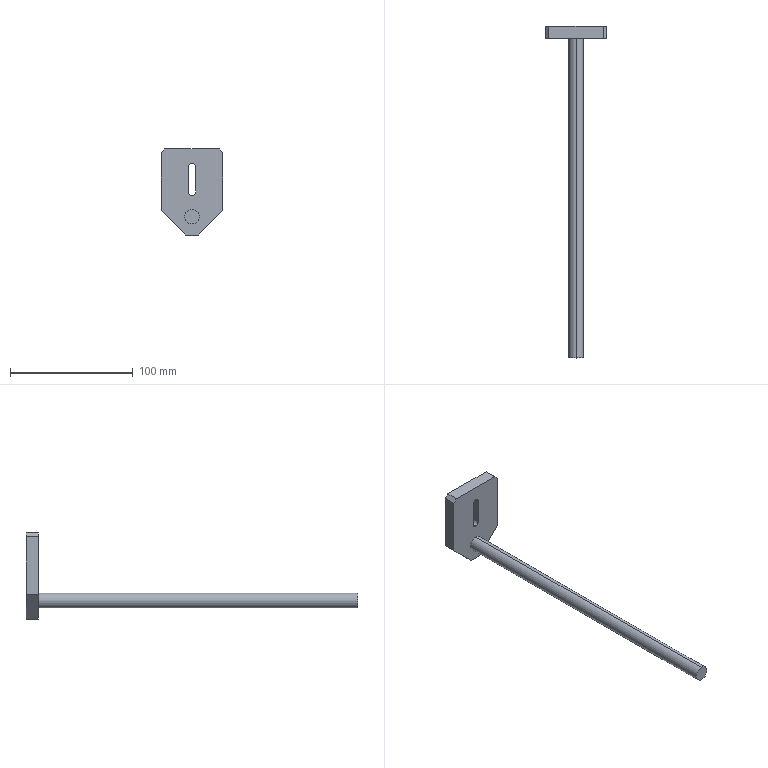Part | SolidWorks | features ICE 2, Chamfer 1, Extrusion 1, HoleWzd 1 | 1 solid | 20 faces | box 50 x 270 x 70 mm | volume 58386 mm3 | plane 13 | cylinder 7 | commonest cylinder face diameters 6 x3 4.2 x2 12 x2
STEP:
#1=CARTESIAN_POINT('',(0.,10.,-13.));
#2=VERTEX_POINT('',#1);
#3=CARTESIAN_POINT('',(3.,10.,-10.));
#4=VERTEX_POINT('',#3);
#5=CARTESIAN_POINT('',(0.,10.,-10.));
#6=DIRECTION('',(0.,-1.,0.));
#7=DIRECTION('',(0.,0.,-1.));
#8=AXIS2_PLACEMENT_3D('',#5,#6,#7);
#9=CIRCLE('',#8,3.);
#10=EDGE_CURVE('',#2,#4,#9,.T.);
#11=ORIENTED_EDGE('',*,*,#10,.F.);
#12=CARTESIAN_POINT('',(0.,7.1,-13.));
#13=VERTEX_POINT('',#12);
#14=CARTESIAN_POINT('',(0.,10.,-13.));
#15=DIRECTION('',(0.,-1.,0.));
#16=VECTOR('',#15,1000.);
#17=LINE('',#14,#16);
#18=EDGE_CURVE('',#2,#13,#17,.T.);
#19=ORIENTED_EDGE('',*,*,#18,.T.);
#20=CARTESIAN_POINT('',(2.1,5.,-12.142));
#21=VERTEX_POINT('',#20);
#22=CARTESIAN_POINT('',(2.1,5.,-12.142));
#23=CARTESIAN_POINT('',(2.1,5.142,-12.142));
#24=CARTESIAN_POINT('',(2.085,5.286,-12.157));
#25=CARTESIAN_POINT('',(2.028,5.562,-12.211));
#26=CARTESIAN_POINT('',(1.986,5.695,-12.249));
#27=CARTESIAN_POINT('',(1.88,5.946,-12.339));
#28=CARTESIAN_POINT('',(1.816,6.063,-12.39));
#29=CARTESIAN_POINT('',(1.668,6.282,-12.495));
#30=CARTESIAN_POINT('',(1.583,6.386,-12.551));
#31=CARTESIAN_POINT('',(1.396,6.574,-12.657));
#32=CARTESIAN_POINT('',(1.295,6.659,-12.709));
#33=CARTESIAN_POINT('',(1.072,6.811,-12.804));
#34=CARTESIAN_POINT('',(0.9508,6.877,-12.848));
#35=CARTESIAN_POINT('',(0.6972,6.986,-12.921));
#36=CARTESIAN_POINT('',(0.5628,7.028,-12.95));
#37=CARTESIAN_POINT('',(0.2837,7.086,-12.99));
#38=CARTESIAN_POINT('',(0.1426,7.1,-13.));
#39=CARTESIAN_POINT('',(0.,7.1,-13.));
#40=B_SPLINE_CURVE_WITH_KNOTS('',3,(#22,#23,#24,#25,#26,#27,#28,#29,#30,#31,#32,#33,#34,#35,#36,#37,#38,#39),.UNSPECIFIED.,.F.,.F.,(4,2,2,2,2,2,2,2,4),(0.006811,0.007236,0.007662,0.008087,0.008512,0.008938,0.009363,0.009789,0.01021),.UNSPECIFIED.);
#41=EDGE_CURVE('',#21,#13,#40,.T.);
#42=ORIENTED_EDGE('',*,*,#41,.F.);
#43=CARTESIAN_POINT('',(0.,2.9,-13.));
#44=VERTEX_POINT('',#43);
#45=CARTESIAN_POINT('',(0.,2.9,-13.));
#46=CARTESIAN_POINT('',(0.1432,2.9,-13.));
#47=CARTESIAN_POINT('',(0.2844,2.914,-12.99));
#48=CARTESIAN_POINT('',(0.5628,2.972,-12.95));
#49=CARTESIAN_POINT('',(0.6977,3.014,-12.921));
#50=CARTESIAN_POINT('',(0.9516,3.123,-12.848));
#51=CARTESIAN_POINT('',(1.073,3.19,-12.804));
#52=CARTESIAN_POINT('',(1.295,3.342,-12.709));
#53=CARTESIAN_POINT('',(1.397,3.427,-12.657));
#54=CARTESIAN_POINT('',(1.679,3.711,-12.495));
#55=CARTESIAN_POINT('',(1.828,3.93,-12.383));
#56=CARTESIAN_POINT('',(1.987,4.308,-12.249));
#57=CARTESIAN_POINT('',(2.028,4.439,-12.211));
#58=CARTESIAN_POINT('',(2.085,4.715,-12.157));
#59=CARTESIAN_POINT('',(2.1,4.858,-12.142));
#60=CARTESIAN_POINT('',(2.1,5.,-12.142));
#61=B_SPLINE_CURVE_WITH_KNOTS('',3,(#45,#46,#47,#48,#49,#50,#51,#52,#53,#54,#55,#56,#57,#58,#59,#60),.UNSPECIFIED.,.F.,.F.,(4,2,2,2,2,2,2,4),(0.003408,0.003833,0.004259,0.004684,0.005109,0.00596,0.006386,0.006811),.UNSPECIFIED.);
#62=EDGE_CURVE('',#44,#21,#61,.T.);
#63=ORIENTED_EDGE('',*,*,#62,.F.);
#64=CARTESIAN_POINT('',(0.,0.,-13.));
#65=VERTEX_POINT('',#64);
#66=CARTESIAN_POINT('',(0.,10.,-13.));
#67=DIRECTION('',(0.,-1.,0.));
#68=VECTOR('',#67,1000.);
#69=LINE('',#66,#68);
#70=EDGE_CURVE('',#44,#65,#69,.T.);
#71=ORIENTED_EDGE('',*,*,#70,.T.);
#72=CARTESIAN_POINT('',(3.,0.,-10.));
#73=VERTEX_POINT('',#72);
#74=CARTESIAN_POINT('',(0.,0.,-10.));
#75=DIRECTION('',(0.,-1.,0.));
#76=DIRECTION('',(0.,0.,-1.));
#77=AXIS2_PLACEMENT_3D('',#74,#75,#76);
#78=CIRCLE('',#77,3.);
#79=EDGE_CURVE('',#65,#73,#78,.T.);
#80=ORIENTED_EDGE('',*,*,#79,.T.);
#81=CARTESIAN_POINT('',(3.,10.,-10.));
#82=DIRECTION('',(0.,-1.,0.));
#83=VECTOR('',#82,1000.);
#84=LINE('',#81,#83);
#85=EDGE_CURVE('',#4,#73,#84,.T.);
#86=ORIENTED_EDGE('',*,*,#85,.F.);
#87=EDGE_LOOP('',(#11,#19,#42,#63,#71,#80,#86));
#88=FACE_OUTER_BOUND('',#87,.T.);
#89=CARTESIAN_POINT('',(0.,10.,-10.));
#90=DIRECTION('',(0.,-1.,0.));
#91=DIRECTION('',(0.,0.,-1.));
#92=AXIS2_PLACEMENT_3D('',#89,#90,#91);
#93=CYLINDRICAL_SURFACE('',#92,3.);
#94=ADVANCED_FACE('',(#88),#93,.F.);
#95=CARTESIAN_POINT('',(-2.1,5.,-12.142));
#96=VERTEX_POINT('',#95);
#97=CARTESIAN_POINT('',(-2.1,5.,-12.142));
#98=CARTESIAN_POINT('',(-2.1,4.855,-12.142));
#99=CARTESIAN_POINT('',(-2.085,4.715,-12.157));
#100=CARTESIAN_POINT('',(-2.029,4.44,-12.21));
#101=CARTESIAN_POINT('',(-1.987,4.306,-12.249));
#102=CARTESIAN_POINT('',(-1.828,3.932,-12.383));
#103=CARTESIAN_POINT('',(-1.677,3.709,-12.497));
#104=CARTESIAN_POINT('',(-1.397,3.427,-12.657));
#105=CARTESIAN_POINT('',(-1.293,3.34,-12.71));
#106=CARTESIAN_POINT('',(-1.072,3.189,-12.805));
#107=CARTESIAN_POINT('',(-0.9538,3.124,-12.847));
#108=CARTESIAN_POINT('',(-0.7002,3.015,-12.92));
#109=CARTESIAN_POINT('',(-0.5641,2.972,-12.95));
#110=CARTESIAN_POINT('',(-0.2875,2.915,-12.989));
#111=CARTESIAN_POINT('',(-0.1435,2.9,-13.));
#112=CARTESIAN_POINT('',(0.,2.9,-13.));
#113=B_SPLINE_CURVE_WITH_KNOTS('',3,(#97,#98,#99,#100,#101,#102,#103,#104,#105,#106,#107,#108,#109,#110,#111,#112),.UNSPECIFIED.,.F.,.F.,(4,2,2,2,2,2,2,4),(0.,0.000426,0.000852,0.001704,0.00213,0.002556,0.002982,0.003408),.UNSPECIFIED.);
#114=EDGE_CURVE('',#96,#44,#113,.T.);
#115=ORIENTED_EDGE('',*,*,#114,.T.);
#116=ORIENTED_EDGE('',*,*,#62,.T.);
#117=CARTESIAN_POINT('',(2.1,5.,-45.));
#118=VERTEX_POINT('',#117);
#119=CARTESIAN_POINT('',(2.1,5.,-45.));
#120=DIRECTION('',(0.,0.,-1.));
#121=VECTOR('',#120,1000.);
#122=LINE('',#119,#121);
#123=EDGE_CURVE('',#21,#118,#122,.T.);
#124=ORIENTED_EDGE('',*,*,#123,.T.);
#125=CARTESIAN_POINT('',(-2.1,5.,-45.));
#126=VERTEX_POINT('',#125);
#127=CARTESIAN_POINT('',(0.,5.,-45.));
#128=DIRECTION('',(0.,0.,-1.));
#129=DIRECTION('',(-1.,0.,0.));
#130=AXIS2_PLACEMENT_3D('',#127,#128,#129);
#131=CIRCLE('',#130,2.1);
#132=EDGE_CURVE('',#118,#126,#131,.T.);
#133=ORIENTED_EDGE('',*,*,#132,.T.);
#134=CARTESIAN_POINT('',(-2.1,5.,-45.));
#135=DIRECTION('',(0.,0.,-1.));
#136=VECTOR('',#135,1000.);
#137=LINE('',#134,#136);
#138=EDGE_CURVE('',#96,#126,#137,.T.);
#139=ORIENTED_EDGE('',*,*,#138,.F.);
#140=EDGE_LOOP('',(#115,#116,#124,#133,#139));
#141=FACE_OUTER_BOUND('',#140,.T.);
#142=CARTESIAN_POINT('',(0.,5.,-45.));
#143=DIRECTION('',(0.,0.,-1.));
#144=DIRECTION('',(-1.,0.,0.));
#145=AXIS2_PLACEMENT_3D('',#142,#143,#144);
#146=CYLINDRICAL_SURFACE('',#145,2.1);
#147=ADVANCED_FACE('',(#141),#146,.F.);
#148=CARTESIAN_POINT('',(0.,-260.,-36.));
#149=VERTEX_POINT('',#148);
#150=CARTESIAN_POINT('',(0.,-260.,-24.));
#151=VERTEX_POINT('',#150);
#152=CARTESIAN_POINT('',(0.,-260.,-30.));
#153=DIRECTION('',(0.,-1.,0.));
#154=DIRECTION('',(0.,0.,-1.));
#155=AXIS2_PLACEMENT_3D('',#152,#153,#154);
#156=CIRCLE('',#155,6.);
#157=EDGE_CURVE('',#149,#151,#156,.T.);
#158=ORIENTED_EDGE('',*,*,#157,.F.);
#159=CARTESIAN_POINT('',(0.,0.,-36.));
#160=VERTEX_POINT('',#159);
#161=CARTESIAN_POINT('',(0.,-260.,-36.));
#162=DIRECTION('',(0.,1.,0.));
#163=VECTOR('',#162,1000.);
#164=LINE('',#161,#163);
#165=EDGE_CURVE('',#149,#160,#164,.T.);
#166=ORIENTED_EDGE('',*,*,#165,.T.);
#167=CARTESIAN_POINT('',(0.,0.,-24.));
#168=VERTEX_POINT('',#167);
#169=CARTESIAN_POINT('',(0.,0.,-30.));
#170=DIRECTION('',(0.,-1.,0.));
#171=DIRECTION('',(0.,0.,1.));
#172=AXIS2_PLACEMENT_3D('',#169,#170,#171);
#173=CIRCLE('',#172,6.);
#174=EDGE_CURVE('',#160,#168,#173,.T.);
#175=ORIENTED_EDGE('',*,*,#174,.T.);
#176=CARTESIAN_POINT('',(0.,-260.,-24.));
#177=DIRECTION('',(0.,1.,0.));
#178=VECTOR('',#177,1000.);
#179=LINE('',#176,#178);
#180=EDGE_CURVE('',#151,#168,#179,.T.);
#181=ORIENTED_EDGE('',*,*,#180,.F.);
#182=EDGE_LOOP('',(#158,#166,#175,#181));
#183=FACE_OUTER_BOUND('',#182,.T.);
#184=CARTESIAN_POINT('',(0.,-260.,-30.));
#185=DIRECTION('',(0.,1.,0.));
#186=DIRECTION('',(0.,0.,1.));
#187=AXIS2_PLACEMENT_3D('',#184,#185,#186);
#188=CYLINDRICAL_SURFACE('',#187,6.);
#189=ADVANCED_FACE('',(#183),#188,.T.);
#190=CARTESIAN_POINT('',(25.,0.,-25.));
#191=VERTEX_POINT('',#190);
#192=CARTESIAN_POINT('',(5.,0.,-45.));
#193=VERTEX_POINT('',#192);
#194=CARTESIAN_POINT('',(5.,0.,-45.));
#195=DIRECTION('',(-0.7071,0.,-0.7071));
#196=VECTOR('',#195,1000.);
#197=LINE('',#194,#196);
#198=EDGE_CURVE('',#191,#193,#197,.T.);
#199=ORIENTED_EDGE('',*,*,#198,.T.);
#200=CARTESIAN_POINT('',(5.,10.,-45.));
#201=VERTEX_POINT('',#200);
#202=CARTESIAN_POINT('',(5.,10.,-45.));
#203=DIRECTION('',(0.,-1.,0.));
#204=VECTOR('',#203,1000.);
#205=LINE('',#202,#204);
#206=EDGE_CURVE('',#201,#193,#205,.T.);
#207=ORIENTED_EDGE('',*,*,#206,.F.);
#208=CARTESIAN_POINT('',(25.,10.,-25.));
#209=VERTEX_POINT('',#208);
#210=CARTESIAN_POINT('',(5.,10.,-45.));
#211=DIRECTION('',(-0.7071,0.,-0.7071));
#212=VECTOR('',#211,1000.);
#213=LINE('',#210,#212);
#214=EDGE_CURVE('',#209,#201,#213,.T.);
#215=ORIENTED_EDGE('',*,*,#214,.F.);
#216=CARTESIAN_POINT('',(25.,10.,-25.));
#217=DIRECTION('',(0.,-1.,0.));
#218=VECTOR('',#217,1000.);
#219=LINE('',#216,#218);
#220=EDGE_CURVE('',#209,#191,#219,.T.);
#221=ORIENTED_EDGE('',*,*,#220,.T.);
#222=EDGE_LOOP('',(#199,#207,#215,#221));
#223=FACE_OUTER_BOUND('',#222,.T.);
#224=CARTESIAN_POINT('',(5.,10.,-45.));
#225=DIRECTION('',(-0.7071,0.,0.7071));
#226=DIRECTION('',(0.7071,0.,0.7071));
#227=AXIS2_PLACEMENT_3D('',#224,#225,#226);
#228=PLANE('',#227);
#229=ADVANCED_FACE('',(#223),#228,.F.);
#230=CARTESIAN_POINT('',(0.,5.,-45.));
#231=DIRECTION('',(0.,0.,-1.));
#232=DIRECTION('',(-1.,0.,0.));
#233=AXIS2_PLACEMENT_3D('',#230,#231,#232);
#234=CIRCLE('',#233,2.1);
#235=EDGE_CURVE('',#126,#118,#234,.T.);
#236=ORIENTED_EDGE('',*,*,#235,.F.);
#237=ORIENTED_EDGE('',*,*,#132,.F.);
#238=EDGE_LOOP('',(#236,#237));
#239=FACE_BOUND('',#238,.T.);
#240=CARTESIAN_POINT('',(-5.,0.,-45.));
#241=VERTEX_POINT('',#240);
#242=CARTESIAN_POINT('',(-5.,0.,-45.));
#243=DIRECTION('',(-1.,0.,0.));
#244=VECTOR('',#243,1000.);
#245=LINE('',#242,#244);
#246=EDGE_CURVE('',#193,#241,#245,.T.);
#247=ORIENTED_EDGE('',*,*,#246,.T.);
#248=CARTESIAN_POINT('',(-5.,10.,-45.));
#249=VERTEX_POINT('',#248);
#250=CARTESIAN_POINT('',(-5.,10.,-45.));
#251=DIRECTION('',(0.,-1.,0.));
#252=VECTOR('',#251,1000.);
#253=LINE('',#250,#252);
#254=EDGE_CURVE('',#249,#241,#253,.T.);
#255=ORIENTED_EDGE('',*,*,#254,.F.);
#256=CARTESIAN_POINT('',(-5.,10.,-45.));
#257=DIRECTION('',(-1.,0.,0.));
#258=VECTOR('',#257,1000.);
#259=LINE('',#256,#258);
#260=EDGE_CURVE('',#201,#249,#259,.T.);
#261=ORIENTED_EDGE('',*,*,#260,.F.);
#262=ORIENTED_EDGE('',*,*,#206,.T.);
#263=EDGE_LOOP('',(#247,#255,#261,#262));
#264=FACE_OUTER_BOUND('',#263,.T.);
#265=CARTESIAN_POINT('',(-5.,10.,-45.));
#266=DIRECTION('',(0.,0.,1.));
#267=DIRECTION('',(1.,0.,0.));
#268=AXIS2_PLACEMENT_3D('',#265,#266,#267);
#269=PLANE('',#268);
#270=ADVANCED_FACE('',(#239,#264),#269,.F.);
#271=CARTESIAN_POINT('',(-25.,0.,-25.));
#272=VERTEX_POINT('',#271);
#273=CARTESIAN_POINT('',(-25.,0.,-25.));
#274=DIRECTION('',(-0.7071,0.,0.7071));
#275=VECTOR('',#274,1000.);
#276=LINE('',#273,#275);
#277=EDGE_CURVE('',#241,#272,#276,.T.);
#278=ORIENTED_EDGE('',*,*,#277,.T.);
#279=CARTESIAN_POINT('',(-25.,10.,-25.));
#280=VERTEX_POINT('',#279);
#281=CARTESIAN_POINT('',(-25.,10.,-25.));
#282=DIRECTION('',(0.,-1.,0.));
#283=VECTOR('',#282,1000.);
#284=LINE('',#281,#283);
#285=EDGE_CURVE('',#280,#272,#284,.T.);
#286=ORIENTED_EDGE('',*,*,#285,.F.);
#287=CARTESIAN_POINT('',(-25.,10.,-25.));
#288=DIRECTION('',(-0.7071,0.,0.7071));
#289=VECTOR('',#288,1000.);
#290=LINE('',#287,#289);
#291=EDGE_CURVE('',#249,#280,#290,.T.);
#292=ORIENTED_EDGE('',*,*,#291,.F.);
#293=ORIENTED_EDGE('',*,*,#254,.T.);
#294=EDGE_LOOP('',(#278,#286,#292,#293));
#295=FACE_OUTER_BOUND('',#294,.T.);
#296=CARTESIAN_POINT('',(-25.,10.,-25.));
#297=DIRECTION('',(0.7071,0.,0.7071));
#298=DIRECTION('',(0.7071,0.,-0.7071));
#299=AXIS2_PLACEMENT_3D('',#296,#297,#298);
#300=PLANE('',#299);
#301=ADVANCED_FACE('',(#295),#300,.F.);
#302=CARTESIAN_POINT('',(-25.,0.,22.));
#303=VERTEX_POINT('',#302);
#304=CARTESIAN_POINT('',(-25.,0.,25.));
#305=DIRECTION('',(0.,0.,1.));
#306=VECTOR('',#305,1000.);
#307=LINE('',#304,#306);
#308=EDGE_CURVE('',#272,#303,#307,.T.);
#309=ORIENTED_EDGE('',*,*,#308,.T.);
#310=CARTESIAN_POINT('',(-25.,10.,22.));
#311=VERTEX_POINT('',#310);
#312=CARTESIAN_POINT('',(-25.,10.,22.));
#313=DIRECTION('',(0.,1.,0.));
#314=VECTOR('',#313,1000.);
#315=LINE('',#312,#314);
#316=EDGE_CURVE('',#303,#311,#315,.T.);
#317=ORIENTED_EDGE('',*,*,#316,.T.);
#318=CARTESIAN_POINT('',(-25.,10.,25.));
#319=DIRECTION('',(0.,0.,1.));
#320=VECTOR('',#319,1000.);
#321=LINE('',#318,#320);
#322=EDGE_CURVE('',#280,#311,#321,.T.);
#323=ORIENTED_EDGE('',*,*,#322,.F.);
#324=ORIENTED_EDGE('',*,*,#285,.T.);
#325=EDGE_LOOP('',(#309,#317,#323,#324));
#326=FACE_OUTER_BOUND('',#325,.T.);
#327=CARTESIAN_POINT('',(-25.,10.,25.));
#328=DIRECTION('',(1.,0.,0.));
#329=DIRECTION('',(0.,0.,-1.));
#330=AXIS2_PLACEMENT_3D('',#327,#328,#329);
#331=PLANE('',#330);
#332=ADVANCED_FACE('',(#326),#331,.F.);
#333=CARTESIAN_POINT('',(-22.,0.,25.));
#334=VERTEX_POINT('',#333);
#335=CARTESIAN_POINT('',(22.,0.,25.));
#336=VERTEX_POINT('',#335);
#337=CARTESIAN_POINT('',(-25.,0.,25.));
#338=DIRECTION('',(1.,0.,0.));
#339=VECTOR('',#338,1000.);
#340=LINE('',#337,#339);
#341=EDGE_CURVE('',#334,#336,#340,.T.);
#342=ORIENTED_EDGE('',*,*,#341,.T.);
#343=CARTESIAN_POINT('',(22.,10.,25.));
#344=VERTEX_POINT('',#343);
#345=CARTESIAN_POINT('',(22.,10.,25.));
#346=DIRECTION('',(0.,1.,0.));
#347=VECTOR('',#346,1000.);
#348=LINE('',#345,#347);
#349=EDGE_CURVE('',#336,#344,#348,.T.);
#350=ORIENTED_EDGE('',*,*,#349,.T.);
#351=CARTESIAN_POINT('',(-22.,10.,25.));
#352=VERTEX_POINT('',#351);
#353=CARTESIAN_POINT('',(-25.,10.,25.));
#354=DIRECTION('',(1.,0.,0.));
#355=VECTOR('',#354,1000.);
#356=LINE('',#353,#355);
#357=EDGE_CURVE('',#352,#344,#356,.T.);
#358=ORIENTED_EDGE('',*,*,#357,.F.);
#359=CARTESIAN_POINT('',(-22.,10.,25.));
#360=DIRECTION('',(0.,-1.,0.));
#361=VECTOR('',#360,1000.);
#362=LINE('',#359,#361);
#363=EDGE_CURVE('',#352,#334,#362,.T.);
#364=ORIENTED_EDGE('',*,*,#363,.T.);
#365=EDGE_LOOP('',(#342,#350,#358,#364));
#366=FACE_OUTER_BOUND('',#365,.T.);
#367=CARTESIAN_POINT('',(-25.,10.,25.));
#368=DIRECTION('',(0.,0.,-1.));
#369=DIRECTION('',(-1.,0.,0.));
#370=AXIS2_PLACEMENT_3D('',#367,#368,#369);
#371=PLANE('',#370);
#372=ADVANCED_FACE('',(#366),#371,.F.);
#373=CARTESIAN_POINT('',(25.,10.,22.));
#374=VERTEX_POINT('',#373);
#375=CARTESIAN_POINT('',(25.,10.,25.));
#376=DIRECTION('',(0.,0.,-1.));
#377=VECTOR('',#376,1000.);
#378=LINE('',#375,#377);
#379=EDGE_CURVE('',#374,#209,#378,.T.);
#380=ORIENTED_EDGE('',*,*,#379,.F.);
#381=CARTESIAN_POINT('',(25.,0.,22.));
#382=VERTEX_POINT('',#381);
#383=CARTESIAN_POINT('',(25.,10.,22.));
#384=DIRECTION('',(0.,-1.,0.));
#385=VECTOR('',#384,1000.);
#386=LINE('',#383,#385);
#387=EDGE_CURVE('',#374,#382,#386,.T.);
#388=ORIENTED_EDGE('',*,*,#387,.T.);
#389=CARTESIAN_POINT('',(25.,0.,25.));
#390=DIRECTION('',(0.,0.,-1.));
#391=VECTOR('',#390,1000.);
#392=LINE('',#389,#391);
#393=EDGE_CURVE('',#382,#191,#392,.T.);
#394=ORIENTED_EDGE('',*,*,#393,.T.);
#395=ORIENTED_EDGE('',*,*,#220,.F.);
#396=EDGE_LOOP('',(#380,#388,#394,#395));
#397=FACE_OUTER_BOUND('',#396,.T.);
#398=CARTESIAN_POINT('',(25.,10.,25.));
#399=DIRECTION('',(-1.,0.,0.));
#400=DIRECTION('',(0.,0.,1.));
#401=AXIS2_PLACEMENT_3D('',#398,#399,#400);
#402=PLANE('',#401);
#403=ADVANCED_FACE('',(#397),#402,.F.);
#404=CARTESIAN_POINT('',(3.,10.,10.));
#405=VERTEX_POINT('',#404);
#406=CARTESIAN_POINT('',(-3.,10.,10.));
#407=VERTEX_POINT('',#406);
#408=CARTESIAN_POINT('',(0.,10.,10.));
#409=DIRECTION('',(0.,-1.,0.));
#410=DIRECTION('',(0.,0.,-1.));
#411=AXIS2_PLACEMENT_3D('',#408,#409,#410);
#412=CIRCLE('',#411,3.);
#413=EDGE_CURVE('',#405,#407,#412,.T.);
#414=ORIENTED_EDGE('',*,*,#413,.T.);
#415=CARTESIAN_POINT('',(-3.,10.,-10.));
#416=VERTEX_POINT('',#415);
#417=CARTESIAN_POINT('',(-3.,10.,10.));
#418=DIRECTION('',(0.,0.,-1.));
#419=VECTOR('',#418,1000.);
#420=LINE('',#417,#419);
#421=EDGE_CURVE('',#407,#416,#420,.T.);
#422=ORIENTED_EDGE('',*,*,#421,.T.);
#423=CARTESIAN_POINT('',(0.,10.,-10.));
#424=DIRECTION('',(0.,-1.,0.));
#425=DIRECTION('',(0.,0.,-1.));
#426=AXIS2_PLACEMENT_3D('',#423,#424,#425);
#427=CIRCLE('',#426,3.);
#428=EDGE_CURVE('',#416,#2,#427,.T.);
#429=ORIENTED_EDGE('',*,*,#428,.T.);
#430=ORIENTED_EDGE('',*,*,#10,.T.);
#431=CARTESIAN_POINT('',(3.,10.,10.));
#432=DIRECTION('',(0.,0.,1.));
#433=VECTOR('',#432,1000.);
#434=LINE('',#431,#433);
#435=EDGE_CURVE('',#4,#405,#434,.T.);
#436=ORIENTED_EDGE('',*,*,#435,.T.);
#437=EDGE_LOOP('',(#414,#422,#429,#430,#436));
#438=FACE_BOUND('',#437,.T.);
#439=ORIENTED_EDGE('',*,*,#357,.T.);
#440=CARTESIAN_POINT('',(23.5,10.,23.5));
#441=DIRECTION('',(0.7071,0.,-0.7071));
#442=VECTOR('',#441,1000.);
#443=LINE('',#440,#442);
#444=EDGE_CURVE('',#344,#374,#443,.T.);
#445=ORIENTED_EDGE('',*,*,#444,.T.);
#446=ORIENTED_EDGE('',*,*,#379,.T.);
#447=ORIENTED_EDGE('',*,*,#214,.T.);
#448=ORIENTED_EDGE('',*,*,#260,.T.);
#449=ORIENTED_EDGE('',*,*,#291,.T.);
#450=ORIENTED_EDGE('',*,*,#322,.T.);
#451=CARTESIAN_POINT('',(-23.5,10.,23.5));
#452=DIRECTION('',(0.7071,0.,0.7071));
#453=VECTOR('',#452,1000.);
#454=LINE('',#451,#453);
#455=EDGE_CURVE('',#311,#352,#454,.T.);
#456=ORIENTED_EDGE('',*,*,#455,.T.);
#457=EDGE_LOOP('',(#439,#445,#446,#447,#448,#449,#450,#456));
#458=FACE_OUTER_BOUND('',#457,.T.);
#459=CARTESIAN_POINT('',(0.,10.,0.));
#460=DIRECTION('',(0.,1.,0.));
#461=DIRECTION('',(0.,0.,1.));
#462=AXIS2_PLACEMENT_3D('',#459,#460,#461);
#463=PLANE('',#462);
#464=ADVANCED_FACE('',(#438,#458),#463,.T.);
#465=CARTESIAN_POINT('',(-3.,0.,10.));
#466=VERTEX_POINT('',#465);
#467=CARTESIAN_POINT('',(-3.,0.,-10.));
#468=VERTEX_POINT('',#467);
#469=CARTESIAN_POINT('',(-3.,0.,10.));
#470=DIRECTION('',(0.,0.,-1.));
#471=VECTOR('',#470,1000.);
#472=LINE('',#469,#471);
#473=EDGE_CURVE('',#466,#468,#472,.T.);
#474=ORIENTED_EDGE('',*,*,#473,.F.);
#475=CARTESIAN_POINT('',(3.,0.,10.));
#476=VERTEX_POINT('',#475);
#477=CARTESIAN_POINT('',(0.,0.,10.));
#478=DIRECTION('',(0.,-1.,0.));
#479=DIRECTION('',(0.,0.,-1.));
#480=AXIS2_PLACEMENT_3D('',#477,#478,#479);
#481=CIRCLE('',#480,3.);
#482=EDGE_CURVE('',#476,#466,#481,.T.);
#483=ORIENTED_EDGE('',*,*,#482,.F.);
#484=CARTESIAN_POINT('',(3.,0.,10.));
#485=DIRECTION('',(0.,0.,1.));
#486=VECTOR('',#485,1000.);
#487=LINE('',#484,#486);
#488=EDGE_CURVE('',#73,#476,#487,.T.);
#489=ORIENTED_EDGE('',*,*,#488,.F.);
#490=ORIENTED_EDGE('',*,*,#79,.F.);
#491=CARTESIAN_POINT('',(0.,0.,-10.));
#492=DIRECTION('',(0.,-1.,0.));
#493=DIRECTION('',(0.,0.,-1.));
#494=AXIS2_PLACEMENT_3D('',#491,#492,#493);
#495=CIRCLE('',#494,3.);
#496=EDGE_CURVE('',#468,#65,#495,.T.);
#497=ORIENTED_EDGE('',*,*,#496,.F.);
#498=EDGE_LOOP('',(#474,#483,#489,#490,#497));
#499=FACE_BOUND('',#498,.T.);
#500=CARTESIAN_POINT('',(0.,0.,-30.));
#501=DIRECTION('',(0.,-1.,0.));
#502=DIRECTION('',(0.,0.,1.));
#503=AXIS2_PLACEMENT_3D('',#500,#501,#502);
#504=CIRCLE('',#503,6.);
#505=EDGE_CURVE('',#168,#160,#504,.T.);
#506=ORIENTED_EDGE('',*,*,#505,.F.);
#507=ORIENTED_EDGE('',*,*,#174,.F.);
#508=EDGE_LOOP('',(#506,#507));
#509=FACE_BOUND('',#508,.T.);
#510=ORIENTED_EDGE('',*,*,#393,.F.);
#511=CARTESIAN_POINT('',(25.,0.,22.));
#512=DIRECTION('',(-0.7071,0.,0.7071));
#513=VECTOR('',#512,1000.);
#514=LINE('',#511,#513);
#515=EDGE_CURVE('',#382,#336,#514,.T.);
#516=ORIENTED_EDGE('',*,*,#515,.T.);
#517=ORIENTED_EDGE('',*,*,#341,.F.);
#518=CARTESIAN_POINT('',(-22.,0.,25.));
#519=DIRECTION('',(-0.7071,0.,-0.7071));
#520=VECTOR('',#519,1000.);
#521=LINE('',#518,#520);
#522=EDGE_CURVE('',#334,#303,#521,.T.);
#523=ORIENTED_EDGE('',*,*,#522,.T.);
#524=ORIENTED_EDGE('',*,*,#308,.F.);
#525=ORIENTED_EDGE('',*,*,#277,.F.);
#526=ORIENTED_EDGE('',*,*,#246,.F.);
#527=ORIENTED_EDGE('',*,*,#198,.F.);
#528=EDGE_LOOP('',(#510,#516,#517,#523,#524,#525,#526,#527));
#529=FACE_OUTER_BOUND('',#528,.T.);
#530=CARTESIAN_POINT('',(0.,0.,0.));
#531=DIRECTION('',(0.,1.,0.));
#532=DIRECTION('',(0.,0.,1.));
#533=AXIS2_PLACEMENT_3D('',#530,#531,#532);
#534=PLANE('',#533);
#535=ADVANCED_FACE('',(#499,#509,#529),#534,.F.);
#536=ORIENTED_EDGE('',*,*,#165,.F.);
#537=CARTESIAN_POINT('',(0.,-260.,-30.));
#538=DIRECTION('',(0.,-1.,0.));
#539=DIRECTION('',(0.,0.,-1.));
#540=AXIS2_PLACEMENT_3D('',#537,#538,#539);
#541=CIRCLE('',#540,6.);
#542=EDGE_CURVE('',#151,#149,#541,.T.);
#543=ORIENTED_EDGE('',*,*,#542,.F.);
#544=ORIENTED_EDGE('',*,*,#180,.T.);
#545=ORIENTED_EDGE('',*,*,#505,.T.);
#546=EDGE_LOOP('',(#536,#543,#544,#545));
#547=FACE_OUTER_BOUND('',#546,.T.);
#548=CARTESIAN_POINT('',(0.,-260.,-30.));
#549=DIRECTION('',(0.,1.,0.));
#550=DIRECTION('',(0.,0.,1.));
#551=AXIS2_PLACEMENT_3D('',#548,#549,#550);
#552=CYLINDRICAL_SURFACE('',#551,6.);
#553=ADVANCED_FACE('',(#547),#552,.T.);
#554=ORIENTED_EDGE('',*,*,#542,.T.);
#555=ORIENTED_EDGE('',*,*,#157,.T.);
#556=EDGE_LOOP('',(#554,#555));
#557=FACE_OUTER_BOUND('',#556,.T.);
#558=CARTESIAN_POINT('',(0.,-260.,-30.));
#559=DIRECTION('',(0.,-1.,0.));
#560=DIRECTION('',(0.,0.,-1.));
#561=AXIS2_PLACEMENT_3D('',#558,#559,#560);
#562=PLANE('',#561);
#563=ADVANCED_FACE('',(#557),#562,.T.);
#564=ORIENTED_EDGE('',*,*,#123,.F.);
#565=ORIENTED_EDGE('',*,*,#41,.T.);
#566=CARTESIAN_POINT('',(0.,7.1,-13.));
#567=CARTESIAN_POINT('',(-0.1424,7.1,-13.));
#568=CARTESIAN_POINT('',(-0.2871,7.085,-12.989));
#569=CARTESIAN_POINT('',(-0.5634,7.028,-12.95));
#570=CARTESIAN_POINT('',(-0.6985,6.985,-12.921));
#571=CARTESIAN_POINT('',(-1.081,6.822,-12.811));
#572=CARTESIAN_POINT('',(-1.306,6.666,-12.709));
#573=CARTESIAN_POINT('',(-1.678,6.29,-12.496));
#574=CARTESIAN_POINT('',(-1.828,6.067,-12.382));
#575=CARTESIAN_POINT('',(-1.986,5.695,-12.249));
#576=CARTESIAN_POINT('',(-2.028,5.562,-12.211));
#577=CARTESIAN_POINT('',(-2.085,5.286,-12.157));
#578=CARTESIAN_POINT('',(-2.1,5.144,-12.142));
#579=CARTESIAN_POINT('',(-2.1,5.,-12.142));
#580=B_SPLINE_CURVE_WITH_KNOTS('',3,(#566,#567,#568,#569,#570,#571,#572,#573,#574,#575,#576,#577,#578,#579),.UNSPECIFIED.,.F.,.F.,(4,2,2,2,2,2,4),(0.01021,0.01064,0.01106,0.01191,0.01276,0.01319,0.01361),.UNSPECIFIED.);
#581=EDGE_CURVE('',#13,#96,#580,.T.);
#582=ORIENTED_EDGE('',*,*,#581,.T.);
#583=ORIENTED_EDGE('',*,*,#138,.T.);
#584=ORIENTED_EDGE('',*,*,#235,.T.);
#585=EDGE_LOOP('',(#564,#565,#582,#583,#584));
#586=FACE_OUTER_BOUND('',#585,.T.);
#587=CARTESIAN_POINT('',(0.,5.,-45.));
#588=DIRECTION('',(0.,0.,-1.));
#589=DIRECTION('',(-1.,0.,0.));
#590=AXIS2_PLACEMENT_3D('',#587,#588,#589);
#591=CYLINDRICAL_SURFACE('',#590,2.1);
#592=ADVANCED_FACE('',(#586),#591,.F.);
#593=ORIENTED_EDGE('',*,*,#18,.F.);
#594=ORIENTED_EDGE('',*,*,#428,.F.);
#595=CARTESIAN_POINT('',(-3.,10.,-10.));
#596=DIRECTION('',(0.,-1.,0.));
#597=VECTOR('',#596,1000.);
#598=LINE('',#595,#597);
#599=EDGE_CURVE('',#416,#468,#598,.T.);
#600=ORIENTED_EDGE('',*,*,#599,.T.);
#601=ORIENTED_EDGE('',*,*,#496,.T.);
#602=ORIENTED_EDGE('',*,*,#70,.F.);
#603=ORIENTED_EDGE('',*,*,#114,.F.);
#604=ORIENTED_EDGE('',*,*,#581,.F.);
#605=EDGE_LOOP('',(#593,#594,#600,#601,#602,#603,#604));
#606=FACE_OUTER_BOUND('',#605,.T.);
#607=CARTESIAN_POINT('',(0.,10.,-10.));
#608=DIRECTION('',(0.,-1.,0.));
#609=DIRECTION('',(0.,0.,-1.));
#610=AXIS2_PLACEMENT_3D('',#607,#608,#609);
#611=CYLINDRICAL_SURFACE('',#610,3.);
#612=ADVANCED_FACE('',(#606),#611,.F.);
#613=ORIENTED_EDGE('',*,*,#482,.T.);
#614=CARTESIAN_POINT('',(-3.,10.,10.));
#615=DIRECTION('',(0.,-1.,0.));
#616=VECTOR('',#615,1000.);
#617=LINE('',#614,#616);
#618=EDGE_CURVE('',#407,#466,#617,.T.);
#619=ORIENTED_EDGE('',*,*,#618,.F.);
#620=ORIENTED_EDGE('',*,*,#413,.F.);
#621=CARTESIAN_POINT('',(3.,10.,10.));
#622=DIRECTION('',(0.,-1.,0.));
#623=VECTOR('',#622,1000.);
#624=LINE('',#621,#623);
#625=EDGE_CURVE('',#405,#476,#624,.T.);
#626=ORIENTED_EDGE('',*,*,#625,.T.);
#627=EDGE_LOOP('',(#613,#619,#620,#626));
#628=FACE_OUTER_BOUND('',#627,.T.);
#629=CARTESIAN_POINT('',(0.,10.,10.));
#630=DIRECTION('',(0.,-1.,0.));
#631=DIRECTION('',(0.,0.,-1.));
#632=AXIS2_PLACEMENT_3D('',#629,#630,#631);
#633=CYLINDRICAL_SURFACE('',#632,3.);
#634=ADVANCED_FACE('',(#628),#633,.F.);
#635=ORIENTED_EDGE('',*,*,#488,.T.);
#636=ORIENTED_EDGE('',*,*,#625,.F.);
#637=ORIENTED_EDGE('',*,*,#435,.F.);
#638=ORIENTED_EDGE('',*,*,#85,.T.);
#639=EDGE_LOOP('',(#635,#636,#637,#638));
#640=FACE_OUTER_BOUND('',#639,.T.);
#641=CARTESIAN_POINT('',(3.,10.,10.));
#642=DIRECTION('',(1.,0.,0.));
#643=DIRECTION('',(0.,0.,-1.));
#644=AXIS2_PLACEMENT_3D('',#641,#642,#643);
#645=PLANE('',#644);
#646=ADVANCED_FACE('',(#640),#645,.F.);
#647=ORIENTED_EDGE('',*,*,#473,.T.);
#648=ORIENTED_EDGE('',*,*,#599,.F.);
#649=ORIENTED_EDGE('',*,*,#421,.F.);
#650=ORIENTED_EDGE('',*,*,#618,.T.);
#651=EDGE_LOOP('',(#647,#648,#649,#650));
#652=FACE_OUTER_BOUND('',#651,.T.);
#653=CARTESIAN_POINT('',(-3.,10.,10.));
#654=DIRECTION('',(-1.,0.,0.));
#655=DIRECTION('',(0.,0.,1.));
#656=AXIS2_PLACEMENT_3D('',#653,#654,#655);
#657=PLANE('',#656);
#658=ADVANCED_FACE('',(#652),#657,.F.);
#659=ORIENTED_EDGE('',*,*,#444,.F.);
#660=ORIENTED_EDGE('',*,*,#349,.F.);
#661=ORIENTED_EDGE('',*,*,#515,.F.);
#662=ORIENTED_EDGE('',*,*,#387,.F.);
#663=EDGE_LOOP('',(#659,#660,#661,#662));
#664=FACE_OUTER_BOUND('',#663,.T.);
#665=CARTESIAN_POINT('',(25.,10.,22.));
#666=DIRECTION('',(-0.7071,0.,-0.7071));
#667=DIRECTION('',(0.,-1.,0.));
#668=AXIS2_PLACEMENT_3D('',#665,#666,#667);
#669=PLANE('',#668);
#670=ADVANCED_FACE('',(#664),#669,.F.);
#671=ORIENTED_EDGE('',*,*,#455,.F.);
#672=ORIENTED_EDGE('',*,*,#316,.F.);
#673=ORIENTED_EDGE('',*,*,#522,.F.);
#674=ORIENTED_EDGE('',*,*,#363,.F.);
#675=EDGE_LOOP('',(#671,#672,#673,#674));
#676=FACE_OUTER_BOUND('',#675,.T.);
#677=CARTESIAN_POINT('',(-22.,10.,25.));
#678=DIRECTION('',(0.7071,0.,-0.7071));
#679=DIRECTION('',(0.,-1.,0.));
#680=AXIS2_PLACEMENT_3D('',#677,#678,#679);
#681=PLANE('',#680);
#682=ADVANCED_FACE('',(#676),#681,.F.);
#683=CLOSED_SHELL('',(#94,#147,#189,#229,#270,#301,#332,#372,#403,#464,#535,#553,#563,#592,#612,#634,#646,#658,#670,#682));
#684=MANIFOLD_SOLID_BREP('',#683);
#685=CARTESIAN_POINT('',(0.,0.,0.));
#686=DIRECTION('',(0.,0.,1.));
#687=DIRECTION('',(1.,0.,0.));
#688=AXIS2_PLACEMENT_3D('',#685,#686,#687);
#689=(LENGTH_UNIT()NAMED_UNIT(*)SI_UNIT(.MILLI.,.METRE.));
#690=UNCERTAINTY_MEASURE_WITH_UNIT(LENGTH_MEASURE(0.00001),#689,'','');
#691=(NAMED_UNIT(*)PLANE_ANGLE_UNIT()SI_UNIT($,.RADIAN.));
#692=(NAMED_UNIT(*)SI_UNIT($,.STERADIAN.)SOLID_ANGLE_UNIT());
#693=(GEOMETRIC_REPRESENTATION_CONTEXT(3)GLOBAL_UNCERTAINTY_ASSIGNED_CONTEXT((#690))GLOBAL_UNIT_ASSIGNED_CONTEXT((#689,#691,#692))REPRESENTATION_CONTEXT('',''));
#694=ADVANCED_BREP_SHAPE_REPRESENTATION('',(#684,#688),#693);